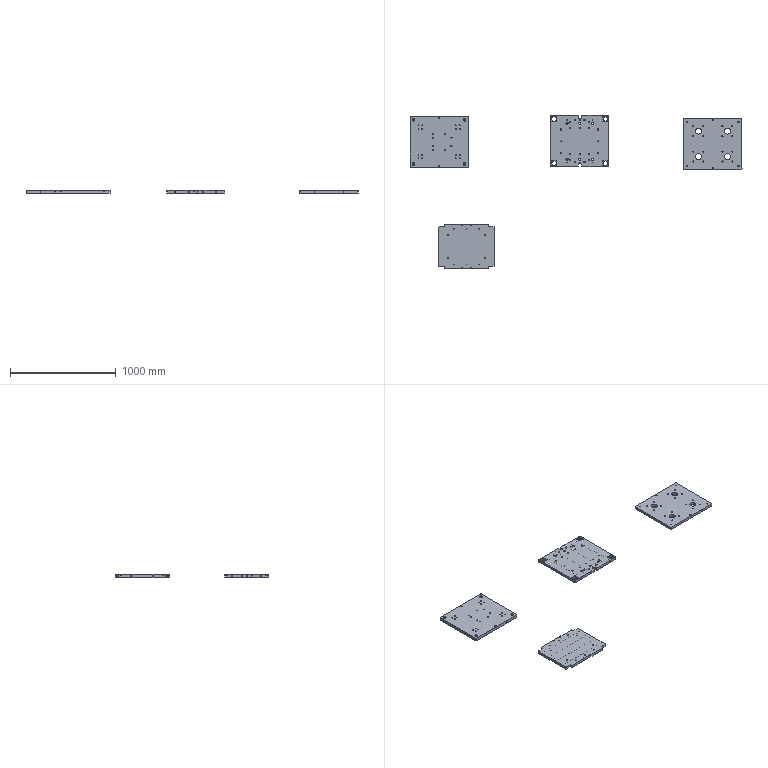NC program | Mastercam | posted with a generic post | part box 3140 x 1452 x 30 mm
Lines 2162 to 2203 of 22248:
N1780 T7 M6
N1790 G0 G90 G17 G54 X276.45 Y-237.1 A0. S6000 M3
N1800 G43 H7 Z50. M8
N1810 Z1.
N1820 G1 Z-.75 F600.
N1830 X276.05 F1000.
N1840 G3 X275.65 Y-237.5 I0. J-.4
N1850 G2 X270. Y-243.15 I-5.65 J0.
N1860 G1 X20.
N1870 G2 X14.35 Y-237.5 I0. J5.65
N1880 G1 Y-225.
N1890 G3 X0. Y-210.65 I-14.35 J0.
N1900 X-14.35 Y-225. I0. J-14.35
N1910 G1 Y-237.5
N1920 G2 X-20. Y-243.15 I-5.65 J0.
N1930 G1 X-270.
N1940 G2 X-275.65 Y-237.5 I0. J5.65
N1950 G3 X-276.05 Y-237.1 I-.4 J0.
N1960 G1 X-276.45
N1970 G0 Z50.
N1980 Y237.1
N1990 Z1.
N2000 G1 Z-.75 F600.
N2010 X-276.05 F1000.
N2020 G3 X-275.65 Y237.5 I0. J.4
N2030 G2 X-270. Y243.15 I5.65 J0.
N2040 G1 X-20.
N2050 G2 X-14.35 Y237.5 I0. J-5.65
N2060 G1 Y225.
N2070 G3 X0. Y210.65 I14.35 J0.
N2080 X14.35 Y225. I0. J14.35
N2090 G1 Y237.5
N2100 G2 X20. Y243.15 I5.65 J0.
N2110 G1 X270.
N2120 G2 X275.65 Y237.5 I0. J-5.65
N2130 G3 X276.05 Y237.1 I.4 J0.
N2140 G1 X276.45
N2150 G0 Z50.
N2160 M5
N2170 G91 G28 Z0. M9
N2180 A0.
N2190 M01